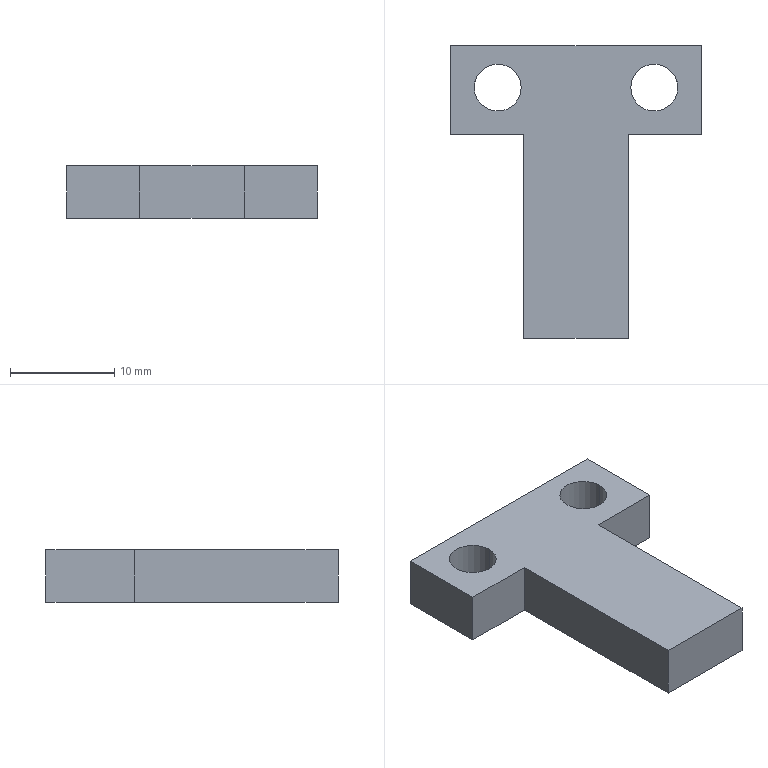Part | STEP file | 11-FG-E04111 | 1 solid | 14 faces | box 24 x 28 x 5 mm | volume 1836 mm3 | plane 10 | cylinder 4 | commonest cylinder face diameters 4.5 x4
STEP:
#1=CARTESIAN_POINT('',(5.25,10.,0.));
#2=VERTEX_POINT('',#1);
#3=CARTESIAN_POINT('',(9.75,10.,0.));
#4=VERTEX_POINT('',#3);
#5=CARTESIAN_POINT('',(7.5,10.,0.));
#6=DIRECTION('',(0.,0.,1.));
#7=DIRECTION('',(1.,0.,0.));
#8=AXIS2_PLACEMENT_3D('',#5,#6,#7);
#9=CIRCLE('',#8,2.25);
#10=EDGE_CURVE('',#2,#4,#9,.T.);
#11=ORIENTED_EDGE('',*,*,#10,.F.);
#12=CARTESIAN_POINT('',(5.25,10.,5.));
#13=VERTEX_POINT('',#12);
#14=CARTESIAN_POINT('',(5.25,10.,-34.));
#15=DIRECTION('',(0.,0.,1.));
#16=VECTOR('',#15,1000.);
#17=LINE('',#14,#16);
#18=EDGE_CURVE('',#2,#13,#17,.T.);
#19=ORIENTED_EDGE('',*,*,#18,.T.);
#20=CARTESIAN_POINT('',(9.75,10.,5.));
#21=VERTEX_POINT('',#20);
#22=CARTESIAN_POINT('',(7.5,10.,5.));
#23=DIRECTION('',(0.,0.,1.));
#24=DIRECTION('',(1.,0.,0.));
#25=AXIS2_PLACEMENT_3D('',#22,#23,#24);
#26=CIRCLE('',#25,2.25);
#27=EDGE_CURVE('',#13,#21,#26,.T.);
#28=ORIENTED_EDGE('',*,*,#27,.T.);
#29=CARTESIAN_POINT('',(9.75,10.,-34.));
#30=DIRECTION('',(0.,0.,1.));
#31=VECTOR('',#30,1000.);
#32=LINE('',#29,#31);
#33=EDGE_CURVE('',#4,#21,#32,.T.);
#34=ORIENTED_EDGE('',*,*,#33,.F.);
#35=EDGE_LOOP('',(#11,#19,#28,#34));
#36=FACE_OUTER_BOUND('',#35,.T.);
#37=CARTESIAN_POINT('',(7.5,10.,-34.));
#38=DIRECTION('',(0.,0.,1.));
#39=DIRECTION('',(1.,0.,0.));
#40=AXIS2_PLACEMENT_3D('',#37,#38,#39);
#41=CYLINDRICAL_SURFACE('',#40,2.25);
#42=ADVANCED_FACE('',(#36),#41,.F.);
#43=CARTESIAN_POINT('',(-9.75,10.,0.));
#44=VERTEX_POINT('',#43);
#45=CARTESIAN_POINT('',(-5.25,10.,0.));
#46=VERTEX_POINT('',#45);
#47=CARTESIAN_POINT('',(-7.5,10.,0.));
#48=DIRECTION('',(0.,0.,1.));
#49=DIRECTION('',(1.,0.,0.));
#50=AXIS2_PLACEMENT_3D('',#47,#48,#49);
#51=CIRCLE('',#50,2.25);
#52=EDGE_CURVE('',#44,#46,#51,.T.);
#53=ORIENTED_EDGE('',*,*,#52,.F.);
#54=CARTESIAN_POINT('',(-9.75,10.,5.));
#55=VERTEX_POINT('',#54);
#56=CARTESIAN_POINT('',(-9.75,10.,-34.));
#57=DIRECTION('',(0.,0.,1.));
#58=VECTOR('',#57,1000.);
#59=LINE('',#56,#58);
#60=EDGE_CURVE('',#44,#55,#59,.T.);
#61=ORIENTED_EDGE('',*,*,#60,.T.);
#62=CARTESIAN_POINT('',(-5.25,10.,5.));
#63=VERTEX_POINT('',#62);
#64=CARTESIAN_POINT('',(-7.5,10.,5.));
#65=DIRECTION('',(0.,0.,1.));
#66=DIRECTION('',(1.,0.,0.));
#67=AXIS2_PLACEMENT_3D('',#64,#65,#66);
#68=CIRCLE('',#67,2.25);
#69=EDGE_CURVE('',#55,#63,#68,.T.);
#70=ORIENTED_EDGE('',*,*,#69,.T.);
#71=CARTESIAN_POINT('',(-5.25,10.,-34.));
#72=DIRECTION('',(0.,0.,1.));
#73=VECTOR('',#72,1000.);
#74=LINE('',#71,#73);
#75=EDGE_CURVE('',#46,#63,#74,.T.);
#76=ORIENTED_EDGE('',*,*,#75,.F.);
#77=EDGE_LOOP('',(#53,#61,#70,#76));
#78=FACE_OUTER_BOUND('',#77,.T.);
#79=CARTESIAN_POINT('',(-7.5,10.,-34.));
#80=DIRECTION('',(0.,0.,1.));
#81=DIRECTION('',(1.,0.,0.));
#82=AXIS2_PLACEMENT_3D('',#79,#80,#81);
#83=CYLINDRICAL_SURFACE('',#82,2.25);
#84=ADVANCED_FACE('',(#78),#83,.F.);
#85=CARTESIAN_POINT('',(-5.,5.5,0.));
#86=VERTEX_POINT('',#85);
#87=CARTESIAN_POINT('',(-5.,5.5,5.));
#88=VERTEX_POINT('',#87);
#89=CARTESIAN_POINT('',(-5.,5.5,-11.011));
#90=DIRECTION('',(0.,0.,1.));
#91=VECTOR('',#90,1000.);
#92=LINE('',#89,#91);
#93=EDGE_CURVE('',#86,#88,#92,.T.);
#94=ORIENTED_EDGE('',*,*,#93,.F.);
#95=CARTESIAN_POINT('',(-5.,-14.,0.));
#96=VERTEX_POINT('',#95);
#97=CARTESIAN_POINT('',(-5.,14.,0.));
#98=DIRECTION('',(0.,-1.,0.));
#99=VECTOR('',#98,1000.);
#100=LINE('',#97,#99);
#101=EDGE_CURVE('',#86,#96,#100,.T.);
#102=ORIENTED_EDGE('',*,*,#101,.T.);
#103=CARTESIAN_POINT('',(-5.,-14.,5.));
#104=VERTEX_POINT('',#103);
#105=CARTESIAN_POINT('',(-5.,-14.,5.));
#106=DIRECTION('',(0.,0.,-1.));
#107=VECTOR('',#106,1000.);
#108=LINE('',#105,#107);
#109=EDGE_CURVE('',#104,#96,#108,.T.);
#110=ORIENTED_EDGE('',*,*,#109,.F.);
#111=CARTESIAN_POINT('',(-5.,14.,5.));
#112=DIRECTION('',(0.,-1.,0.));
#113=VECTOR('',#112,1000.);
#114=LINE('',#111,#113);
#115=EDGE_CURVE('',#88,#104,#114,.T.);
#116=ORIENTED_EDGE('',*,*,#115,.F.);
#117=EDGE_LOOP('',(#94,#102,#110,#116));
#118=FACE_OUTER_BOUND('',#117,.T.);
#119=CARTESIAN_POINT('',(-5.,14.,5.));
#120=DIRECTION('',(1.,0.,0.));
#121=DIRECTION('',(0.,1.,0.));
#122=AXIS2_PLACEMENT_3D('',#119,#120,#121);
#123=PLANE('',#122);
#124=ADVANCED_FACE('',(#118),#123,.F.);
#125=CARTESIAN_POINT('',(5.,-14.,0.));
#126=VERTEX_POINT('',#125);
#127=CARTESIAN_POINT('',(5.,5.5,0.));
#128=VERTEX_POINT('',#127);
#129=CARTESIAN_POINT('',(5.,14.,0.));
#130=DIRECTION('',(0.,1.,0.));
#131=VECTOR('',#130,1000.);
#132=LINE('',#129,#131);
#133=EDGE_CURVE('',#126,#128,#132,.T.);
#134=ORIENTED_EDGE('',*,*,#133,.T.);
#135=CARTESIAN_POINT('',(5.,5.5,5.));
#136=VERTEX_POINT('',#135);
#137=CARTESIAN_POINT('',(5.,5.5,-11.011));
#138=DIRECTION('',(0.,0.,1.));
#139=VECTOR('',#138,1000.);
#140=LINE('',#137,#139);
#141=EDGE_CURVE('',#128,#136,#140,.T.);
#142=ORIENTED_EDGE('',*,*,#141,.T.);
#143=CARTESIAN_POINT('',(5.,-14.,5.));
#144=VERTEX_POINT('',#143);
#145=CARTESIAN_POINT('',(5.,14.,5.));
#146=DIRECTION('',(0.,1.,0.));
#147=VECTOR('',#146,1000.);
#148=LINE('',#145,#147);
#149=EDGE_CURVE('',#144,#136,#148,.T.);
#150=ORIENTED_EDGE('',*,*,#149,.F.);
#151=CARTESIAN_POINT('',(5.,-14.,5.));
#152=DIRECTION('',(0.,0.,-1.));
#153=VECTOR('',#152,1000.);
#154=LINE('',#151,#153);
#155=EDGE_CURVE('',#144,#126,#154,.T.);
#156=ORIENTED_EDGE('',*,*,#155,.T.);
#157=EDGE_LOOP('',(#134,#142,#150,#156));
#158=FACE_OUTER_BOUND('',#157,.T.);
#159=CARTESIAN_POINT('',(5.,14.,5.));
#160=DIRECTION('',(-1.,0.,0.));
#161=DIRECTION('',(0.,-1.,0.));
#162=AXIS2_PLACEMENT_3D('',#159,#160,#161);
#163=PLANE('',#162);
#164=ADVANCED_FACE('',(#158),#163,.F.);
#165=CARTESIAN_POINT('',(12.,14.,0.));
#166=VERTEX_POINT('',#165);
#167=CARTESIAN_POINT('',(-12.,14.,0.));
#168=VERTEX_POINT('',#167);
#169=CARTESIAN_POINT('',(-5.,14.,0.));
#170=DIRECTION('',(-1.,0.,0.));
#171=VECTOR('',#170,1000.);
#172=LINE('',#169,#171);
#173=EDGE_CURVE('',#166,#168,#172,.T.);
#174=ORIENTED_EDGE('',*,*,#173,.T.);
#175=CARTESIAN_POINT('',(-12.,14.,5.));
#176=VERTEX_POINT('',#175);
#177=CARTESIAN_POINT('',(-12.,14.,-11.011));
#178=DIRECTION('',(0.,0.,1.));
#179=VECTOR('',#178,1000.);
#180=LINE('',#177,#179);
#181=EDGE_CURVE('',#168,#176,#180,.T.);
#182=ORIENTED_EDGE('',*,*,#181,.T.);
#183=CARTESIAN_POINT('',(12.,14.,5.));
#184=VERTEX_POINT('',#183);
#185=CARTESIAN_POINT('',(-5.,14.,5.));
#186=DIRECTION('',(-1.,0.,0.));
#187=VECTOR('',#186,1000.);
#188=LINE('',#185,#187);
#189=EDGE_CURVE('',#184,#176,#188,.T.);
#190=ORIENTED_EDGE('',*,*,#189,.F.);
#191=CARTESIAN_POINT('',(12.,14.,-11.011));
#192=DIRECTION('',(0.,0.,1.));
#193=VECTOR('',#192,1000.);
#194=LINE('',#191,#193);
#195=EDGE_CURVE('',#166,#184,#194,.T.);
#196=ORIENTED_EDGE('',*,*,#195,.F.);
#197=EDGE_LOOP('',(#174,#182,#190,#196));
#198=FACE_OUTER_BOUND('',#197,.T.);
#199=CARTESIAN_POINT('',(-5.,14.,5.));
#200=DIRECTION('',(0.,-1.,0.));
#201=DIRECTION('',(0.,0.,-1.));
#202=AXIS2_PLACEMENT_3D('',#199,#200,#201);
#203=PLANE('',#202);
#204=ADVANCED_FACE('',(#198),#203,.F.);
#205=CARTESIAN_POINT('',(-5.,-14.,0.));
#206=DIRECTION('',(1.,0.,0.));
#207=VECTOR('',#206,1000.);
#208=LINE('',#205,#207);
#209=EDGE_CURVE('',#96,#126,#208,.T.);
#210=ORIENTED_EDGE('',*,*,#209,.T.);
#211=ORIENTED_EDGE('',*,*,#155,.F.);
#212=CARTESIAN_POINT('',(-5.,-14.,5.));
#213=DIRECTION('',(1.,0.,0.));
#214=VECTOR('',#213,1000.);
#215=LINE('',#212,#214);
#216=EDGE_CURVE('',#104,#144,#215,.T.);
#217=ORIENTED_EDGE('',*,*,#216,.F.);
#218=ORIENTED_EDGE('',*,*,#109,.T.);
#219=EDGE_LOOP('',(#210,#211,#217,#218));
#220=FACE_OUTER_BOUND('',#219,.T.);
#221=CARTESIAN_POINT('',(-5.,-14.,5.));
#222=DIRECTION('',(0.,1.,0.));
#223=DIRECTION('',(0.,0.,1.));
#224=AXIS2_PLACEMENT_3D('',#221,#222,#223);
#225=PLANE('',#224);
#226=ADVANCED_FACE('',(#220),#225,.F.);
#227=CARTESIAN_POINT('',(7.5,10.,5.));
#228=DIRECTION('',(0.,0.,1.));
#229=DIRECTION('',(1.,0.,0.));
#230=AXIS2_PLACEMENT_3D('',#227,#228,#229);
#231=CIRCLE('',#230,2.25);
#232=EDGE_CURVE('',#21,#13,#231,.T.);
#233=ORIENTED_EDGE('',*,*,#232,.F.);
#234=ORIENTED_EDGE('',*,*,#27,.F.);
#235=EDGE_LOOP('',(#233,#234));
#236=FACE_BOUND('',#235,.T.);
#237=CARTESIAN_POINT('',(-7.5,10.,5.));
#238=DIRECTION('',(0.,0.,1.));
#239=DIRECTION('',(1.,0.,0.));
#240=AXIS2_PLACEMENT_3D('',#237,#238,#239);
#241=CIRCLE('',#240,2.25);
#242=EDGE_CURVE('',#63,#55,#241,.T.);
#243=ORIENTED_EDGE('',*,*,#242,.F.);
#244=ORIENTED_EDGE('',*,*,#69,.F.);
#245=EDGE_LOOP('',(#243,#244));
#246=FACE_BOUND('',#245,.T.);
#247=ORIENTED_EDGE('',*,*,#149,.T.);
#248=CARTESIAN_POINT('',(12.,5.5,5.));
#249=VERTEX_POINT('',#248);
#250=CARTESIAN_POINT('',(5.,5.5,5.));
#251=DIRECTION('',(1.,0.,0.));
#252=VECTOR('',#251,1000.);
#253=LINE('',#250,#252);
#254=EDGE_CURVE('',#136,#249,#253,.T.);
#255=ORIENTED_EDGE('',*,*,#254,.T.);
#256=CARTESIAN_POINT('',(12.,14.,5.));
#257=DIRECTION('',(0.,1.,0.));
#258=VECTOR('',#257,1000.);
#259=LINE('',#256,#258);
#260=EDGE_CURVE('',#249,#184,#259,.T.);
#261=ORIENTED_EDGE('',*,*,#260,.T.);
#262=ORIENTED_EDGE('',*,*,#189,.T.);
#263=CARTESIAN_POINT('',(-12.,5.5,5.));
#264=VERTEX_POINT('',#263);
#265=CARTESIAN_POINT('',(-12.,14.,5.));
#266=DIRECTION('',(0.,-1.,0.));
#267=VECTOR('',#266,1000.);
#268=LINE('',#265,#267);
#269=EDGE_CURVE('',#176,#264,#268,.T.);
#270=ORIENTED_EDGE('',*,*,#269,.T.);
#271=CARTESIAN_POINT('',(-5.,5.5,5.));
#272=DIRECTION('',(1.,0.,0.));
#273=VECTOR('',#272,1000.);
#274=LINE('',#271,#273);
#275=EDGE_CURVE('',#264,#88,#274,.T.);
#276=ORIENTED_EDGE('',*,*,#275,.T.);
#277=ORIENTED_EDGE('',*,*,#115,.T.);
#278=ORIENTED_EDGE('',*,*,#216,.T.);
#279=EDGE_LOOP('',(#247,#255,#261,#262,#270,#276,#277,#278));
#280=FACE_OUTER_BOUND('',#279,.T.);
#281=CARTESIAN_POINT('',(0.,0.,5.));
#282=DIRECTION('',(0.,0.,1.));
#283=DIRECTION('',(1.,0.,0.));
#284=AXIS2_PLACEMENT_3D('',#281,#282,#283);
#285=PLANE('',#284);
#286=ADVANCED_FACE('',(#236,#246,#280),#285,.T.);
#287=CARTESIAN_POINT('',(7.5,10.,0.));
#288=DIRECTION('',(0.,0.,1.));
#289=DIRECTION('',(1.,0.,0.));
#290=AXIS2_PLACEMENT_3D('',#287,#288,#289);
#291=CIRCLE('',#290,2.25);
#292=EDGE_CURVE('',#4,#2,#291,.T.);
#293=ORIENTED_EDGE('',*,*,#292,.T.);
#294=ORIENTED_EDGE('',*,*,#10,.T.);
#295=EDGE_LOOP('',(#293,#294));
#296=FACE_BOUND('',#295,.T.);
#297=CARTESIAN_POINT('',(-7.5,10.,0.));
#298=DIRECTION('',(0.,0.,1.));
#299=DIRECTION('',(1.,0.,0.));
#300=AXIS2_PLACEMENT_3D('',#297,#298,#299);
#301=CIRCLE('',#300,2.25);
#302=EDGE_CURVE('',#46,#44,#301,.T.);
#303=ORIENTED_EDGE('',*,*,#302,.T.);
#304=ORIENTED_EDGE('',*,*,#52,.T.);
#305=EDGE_LOOP('',(#303,#304));
#306=FACE_BOUND('',#305,.T.);
#307=ORIENTED_EDGE('',*,*,#133,.F.);
#308=ORIENTED_EDGE('',*,*,#209,.F.);
#309=ORIENTED_EDGE('',*,*,#101,.F.);
#310=CARTESIAN_POINT('',(-12.,5.5,0.));
#311=VERTEX_POINT('',#310);
#312=CARTESIAN_POINT('',(-5.,5.5,0.));
#313=DIRECTION('',(-1.,0.,0.));
#314=VECTOR('',#313,1000.);
#315=LINE('',#312,#314);
#316=EDGE_CURVE('',#86,#311,#315,.T.);
#317=ORIENTED_EDGE('',*,*,#316,.T.);
#318=CARTESIAN_POINT('',(-12.,14.,0.));
#319=DIRECTION('',(0.,1.,0.));
#320=VECTOR('',#319,1000.);
#321=LINE('',#318,#320);
#322=EDGE_CURVE('',#311,#168,#321,.T.);
#323=ORIENTED_EDGE('',*,*,#322,.T.);
#324=ORIENTED_EDGE('',*,*,#173,.F.);
#325=CARTESIAN_POINT('',(12.,5.5,0.));
#326=VERTEX_POINT('',#325);
#327=CARTESIAN_POINT('',(12.,14.,0.));
#328=DIRECTION('',(0.,-1.,0.));
#329=VECTOR('',#328,1000.);
#330=LINE('',#327,#329);
#331=EDGE_CURVE('',#166,#326,#330,.T.);
#332=ORIENTED_EDGE('',*,*,#331,.T.);
#333=CARTESIAN_POINT('',(5.,5.5,0.));
#334=DIRECTION('',(-1.,0.,0.));
#335=VECTOR('',#334,1000.);
#336=LINE('',#333,#335);
#337=EDGE_CURVE('',#326,#128,#336,.T.);
#338=ORIENTED_EDGE('',*,*,#337,.T.);
#339=EDGE_LOOP('',(#307,#308,#309,#317,#323,#324,#332,#338));
#340=FACE_OUTER_BOUND('',#339,.T.);
#341=CARTESIAN_POINT('',(0.,0.,0.));
#342=DIRECTION('',(0.,0.,1.));
#343=DIRECTION('',(1.,0.,0.));
#344=AXIS2_PLACEMENT_3D('',#341,#342,#343);
#345=PLANE('',#344);
#346=ADVANCED_FACE('',(#296,#306,#340),#345,.F.);
#347=ORIENTED_EDGE('',*,*,#316,.F.);
#348=ORIENTED_EDGE('',*,*,#93,.T.);
#349=ORIENTED_EDGE('',*,*,#275,.F.);
#350=CARTESIAN_POINT('',(-12.,5.5,-11.011));
#351=DIRECTION('',(0.,0.,1.));
#352=VECTOR('',#351,1000.);
#353=LINE('',#350,#352);
#354=EDGE_CURVE('',#311,#264,#353,.T.);
#355=ORIENTED_EDGE('',*,*,#354,.F.);
#356=EDGE_LOOP('',(#347,#348,#349,#355));
#357=FACE_OUTER_BOUND('',#356,.T.);
#358=CARTESIAN_POINT('',(-5.,5.5,-11.011));
#359=DIRECTION('',(0.,-1.,0.));
#360=DIRECTION('',(0.,0.,-1.));
#361=AXIS2_PLACEMENT_3D('',#358,#359,#360);
#362=PLANE('',#361);
#363=ADVANCED_FACE('',(#357),#362,.T.);
#364=ORIENTED_EDGE('',*,*,#322,.F.);
#365=ORIENTED_EDGE('',*,*,#354,.T.);
#366=ORIENTED_EDGE('',*,*,#269,.F.);
#367=ORIENTED_EDGE('',*,*,#181,.F.);
#368=EDGE_LOOP('',(#364,#365,#366,#367));
#369=FACE_OUTER_BOUND('',#368,.T.);
#370=CARTESIAN_POINT('',(-12.,14.,-11.011));
#371=DIRECTION('',(-1.,0.,0.));
#372=DIRECTION('',(0.,0.,1.));
#373=AXIS2_PLACEMENT_3D('',#370,#371,#372);
#374=PLANE('',#373);
#375=ADVANCED_FACE('',(#369),#374,.T.);
#376=ORIENTED_EDGE('',*,*,#331,.F.);
#377=ORIENTED_EDGE('',*,*,#195,.T.);
#378=ORIENTED_EDGE('',*,*,#260,.F.);
#379=CARTESIAN_POINT('',(12.,5.5,-11.011));
#380=DIRECTION('',(0.,0.,1.));
#381=VECTOR('',#380,1000.);
#382=LINE('',#379,#381);
#383=EDGE_CURVE('',#326,#249,#382,.T.);
#384=ORIENTED_EDGE('',*,*,#383,.F.);
#385=EDGE_LOOP('',(#376,#377,#378,#384));
#386=FACE_OUTER_BOUND('',#385,.T.);
#387=CARTESIAN_POINT('',(12.,14.,-11.011));
#388=DIRECTION('',(1.,0.,0.));
#389=DIRECTION('',(0.,0.,-1.));
#390=AXIS2_PLACEMENT_3D('',#387,#388,#389);
#391=PLANE('',#390);
#392=ADVANCED_FACE('',(#386),#391,.T.);
#393=ORIENTED_EDGE('',*,*,#337,.F.);
#394=ORIENTED_EDGE('',*,*,#383,.T.);
#395=ORIENTED_EDGE('',*,*,#254,.F.);
#396=ORIENTED_EDGE('',*,*,#141,.F.);
#397=EDGE_LOOP('',(#393,#394,#395,#396));
#398=FACE_OUTER_BOUND('',#397,.T.);
#399=CARTESIAN_POINT('',(5.,5.5,-11.011));
#400=DIRECTION('',(0.,-1.,0.));
#401=DIRECTION('',(0.,0.,-1.));
#402=AXIS2_PLACEMENT_3D('',#399,#400,#401);
#403=PLANE('',#402);
#404=ADVANCED_FACE('',(#398),#403,.T.);
#405=ORIENTED_EDGE('',*,*,#60,.F.);
#406=ORIENTED_EDGE('',*,*,#302,.F.);
#407=ORIENTED_EDGE('',*,*,#75,.T.);
#408=ORIENTED_EDGE('',*,*,#242,.T.);
#409=EDGE_LOOP('',(#405,#406,#407,#408));
#410=FACE_OUTER_BOUND('',#409,.T.);
#411=CARTESIAN_POINT('',(-7.5,10.,-34.));
#412=DIRECTION('',(0.,0.,1.));
#413=DIRECTION('',(1.,0.,0.));
#414=AXIS2_PLACEMENT_3D('',#411,#412,#413);
#415=CYLINDRICAL_SURFACE('',#414,2.25);
#416=ADVANCED_FACE('',(#410),#415,.F.);
#417=ORIENTED_EDGE('',*,*,#18,.F.);
#418=ORIENTED_EDGE('',*,*,#292,.F.);
#419=ORIENTED_EDGE('',*,*,#33,.T.);
#420=ORIENTED_EDGE('',*,*,#232,.T.);
#421=EDGE_LOOP('',(#417,#418,#419,#420));
#422=FACE_OUTER_BOUND('',#421,.T.);
#423=CARTESIAN_POINT('',(7.5,10.,-34.));
#424=DIRECTION('',(0.,0.,1.));
#425=DIRECTION('',(1.,0.,0.));
#426=AXIS2_PLACEMENT_3D('',#423,#424,#425);
#427=CYLINDRICAL_SURFACE('',#426,2.25);
#428=ADVANCED_FACE('',(#422),#427,.F.);
#429=CLOSED_SHELL('',(#42,#84,#124,#164,#204,#226,#286,#346,#363,#375,#392,#404,#416,#428));
#430=MANIFOLD_SOLID_BREP('',#429);
#431=CARTESIAN_POINT('',(0.,0.,0.));
#432=DIRECTION('',(0.,0.,1.));
#433=DIRECTION('',(1.,0.,0.));
#434=AXIS2_PLACEMENT_3D('',#431,#432,#433);
#435=(LENGTH_UNIT()NAMED_UNIT(*)SI_UNIT(.MILLI.,.METRE.));
#436=UNCERTAINTY_MEASURE_WITH_UNIT(LENGTH_MEASURE(0.00001),#435,'','');
#437=(NAMED_UNIT(*)PLANE_ANGLE_UNIT()SI_UNIT($,.RADIAN.));
#438=(NAMED_UNIT(*)SI_UNIT($,.STERADIAN.)SOLID_ANGLE_UNIT());
#439=(GEOMETRIC_REPRESENTATION_CONTEXT(3)GLOBAL_UNCERTAINTY_ASSIGNED_CONTEXT((#436))GLOBAL_UNIT_ASSIGNED_CONTEXT((#435,#437,#438))REPRESENTATION_CONTEXT('',''));
#440=ADVANCED_BREP_SHAPE_REPRESENTATION('',(#430,#434),#439);